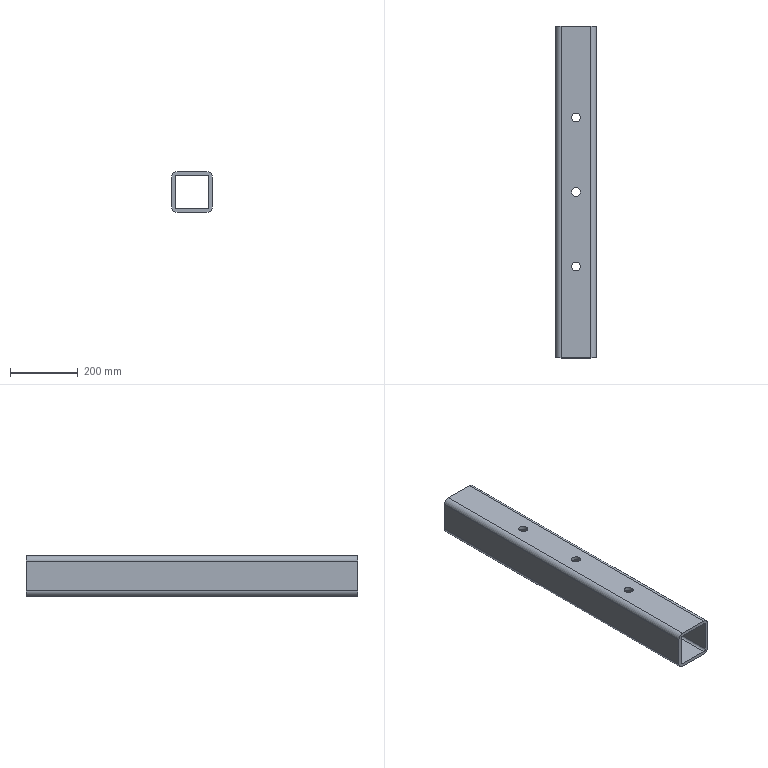Part | SolidWorks | features HoleWzd 1, WeldMemberFeat 1, WeldmentFeature 1 | 1 solid | 30 faces | box 120 x 980 x 120 mm | volume 4095072 mm3 | cylinder 20 | plane 10 | commonest cylinder face diameters 26 x12 12 x4 32 x4
STEP:
#1=CARTESIAN_POINT('',(13.,710.,50.));
#2=VERTEX_POINT('',#1);
#3=CARTESIAN_POINT('',(-13.,710.,50.));
#4=VERTEX_POINT('',#3);
#5=CARTESIAN_POINT('',(0.,710.,50.));
#6=DIRECTION('',(0.,0.,-1.));
#7=DIRECTION('',(-1.,0.,0.));
#8=AXIS2_PLACEMENT_3D('',#5,#6,#7);
#9=CIRCLE('',#8,13.);
#10=EDGE_CURVE('',#2,#4,#9,.T.);
#11=ORIENTED_EDGE('',*,*,#10,.T.);
#12=CARTESIAN_POINT('',(-13.,710.,60.));
#13=VERTEX_POINT('',#12);
#14=CARTESIAN_POINT('',(-13.,710.,60.));
#15=DIRECTION('',(0.,0.,1.));
#16=VECTOR('',#15,1000.);
#17=LINE('',#14,#16);
#18=EDGE_CURVE('',#4,#13,#17,.T.);
#19=ORIENTED_EDGE('',*,*,#18,.T.);
#20=CARTESIAN_POINT('',(13.,710.,60.));
#21=VERTEX_POINT('',#20);
#22=CARTESIAN_POINT('',(0.,710.,60.));
#23=DIRECTION('',(0.,0.,1.));
#24=DIRECTION('',(1.,0.,0.));
#25=AXIS2_PLACEMENT_3D('',#22,#23,#24);
#26=CIRCLE('',#25,13.);
#27=EDGE_CURVE('',#13,#21,#26,.T.);
#28=ORIENTED_EDGE('',*,*,#27,.T.);
#29=CARTESIAN_POINT('',(13.,710.,60.));
#30=DIRECTION('',(0.,0.,1.));
#31=VECTOR('',#30,1000.);
#32=LINE('',#29,#31);
#33=EDGE_CURVE('',#2,#21,#32,.T.);
#34=ORIENTED_EDGE('',*,*,#33,.F.);
#35=EDGE_LOOP('',(#11,#19,#28,#34));
#36=FACE_OUTER_BOUND('',#35,.T.);
#37=CARTESIAN_POINT('',(0.,710.,60.));
#38=DIRECTION('',(0.,0.,1.));
#39=DIRECTION('',(1.,0.,0.));
#40=AXIS2_PLACEMENT_3D('',#37,#38,#39);
#41=CYLINDRICAL_SURFACE('',#40,13.);
#42=ADVANCED_FACE('',(#36),#41,.F.);
#43=CARTESIAN_POINT('',(13.,710.,-60.));
#44=VERTEX_POINT('',#43);
#45=CARTESIAN_POINT('',(-13.,710.,-60.));
#46=VERTEX_POINT('',#45);
#47=CARTESIAN_POINT('',(0.,710.,-60.));
#48=DIRECTION('',(0.,0.,-1.));
#49=DIRECTION('',(1.,0.,0.));
#50=AXIS2_PLACEMENT_3D('',#47,#48,#49);
#51=CIRCLE('',#50,13.);
#52=EDGE_CURVE('',#44,#46,#51,.T.);
#53=ORIENTED_EDGE('',*,*,#52,.T.);
#54=CARTESIAN_POINT('',(-13.,710.,-50.));
#55=VERTEX_POINT('',#54);
#56=CARTESIAN_POINT('',(-13.,710.,60.));
#57=DIRECTION('',(0.,0.,1.));
#58=VECTOR('',#57,1000.);
#59=LINE('',#56,#58);
#60=EDGE_CURVE('',#46,#55,#59,.T.);
#61=ORIENTED_EDGE('',*,*,#60,.T.);
#62=CARTESIAN_POINT('',(13.,710.,-50.));
#63=VERTEX_POINT('',#62);
#64=CARTESIAN_POINT('',(0.,710.,-50.));
#65=DIRECTION('',(0.,0.,1.));
#66=DIRECTION('',(1.,0.,0.));
#67=AXIS2_PLACEMENT_3D('',#64,#65,#66);
#68=CIRCLE('',#67,13.);
#69=EDGE_CURVE('',#55,#63,#68,.T.);
#70=ORIENTED_EDGE('',*,*,#69,.T.);
#71=CARTESIAN_POINT('',(13.,710.,60.));
#72=DIRECTION('',(0.,0.,1.));
#73=VECTOR('',#72,1000.);
#74=LINE('',#71,#73);
#75=EDGE_CURVE('',#44,#63,#74,.T.);
#76=ORIENTED_EDGE('',*,*,#75,.F.);
#77=EDGE_LOOP('',(#53,#61,#70,#76));
#78=FACE_OUTER_BOUND('',#77,.T.);
#79=CARTESIAN_POINT('',(0.,710.,60.));
#80=DIRECTION('',(0.,0.,1.));
#81=DIRECTION('',(1.,0.,0.));
#82=AXIS2_PLACEMENT_3D('',#79,#80,#81);
#83=CYLINDRICAL_SURFACE('',#82,13.);
#84=ADVANCED_FACE('',(#78),#83,.F.);
#85=CARTESIAN_POINT('',(13.,490.,50.));
#86=VERTEX_POINT('',#85);
#87=CARTESIAN_POINT('',(-13.,490.,50.));
#88=VERTEX_POINT('',#87);
#89=CARTESIAN_POINT('',(0.,490.,50.));
#90=DIRECTION('',(0.,0.,-1.));
#91=DIRECTION('',(-1.,0.,0.));
#92=AXIS2_PLACEMENT_3D('',#89,#90,#91);
#93=CIRCLE('',#92,13.);
#94=EDGE_CURVE('',#86,#88,#93,.T.);
#95=ORIENTED_EDGE('',*,*,#94,.T.);
#96=CARTESIAN_POINT('',(-13.,490.,60.));
#97=VERTEX_POINT('',#96);
#98=CARTESIAN_POINT('',(-13.,490.,60.));
#99=DIRECTION('',(0.,0.,1.));
#100=VECTOR('',#99,1000.);
#101=LINE('',#98,#100);
#102=EDGE_CURVE('',#88,#97,#101,.T.);
#103=ORIENTED_EDGE('',*,*,#102,.T.);
#104=CARTESIAN_POINT('',(13.,490.,60.));
#105=VERTEX_POINT('',#104);
#106=CARTESIAN_POINT('',(0.,490.,60.));
#107=DIRECTION('',(0.,0.,1.));
#108=DIRECTION('',(1.,0.,0.));
#109=AXIS2_PLACEMENT_3D('',#106,#107,#108);
#110=CIRCLE('',#109,13.);
#111=EDGE_CURVE('',#97,#105,#110,.T.);
#112=ORIENTED_EDGE('',*,*,#111,.T.);
#113=CARTESIAN_POINT('',(13.,490.,60.));
#114=DIRECTION('',(0.,0.,1.));
#115=VECTOR('',#114,1000.);
#116=LINE('',#113,#115);
#117=EDGE_CURVE('',#86,#105,#116,.T.);
#118=ORIENTED_EDGE('',*,*,#117,.F.);
#119=EDGE_LOOP('',(#95,#103,#112,#118));
#120=FACE_OUTER_BOUND('',#119,.T.);
#121=CARTESIAN_POINT('',(0.,490.,60.));
#122=DIRECTION('',(0.,0.,1.));
#123=DIRECTION('',(1.,0.,0.));
#124=AXIS2_PLACEMENT_3D('',#121,#122,#123);
#125=CYLINDRICAL_SURFACE('',#124,13.);
#126=ADVANCED_FACE('',(#120),#125,.F.);
#127=CARTESIAN_POINT('',(13.,490.,-60.));
#128=VERTEX_POINT('',#127);
#129=CARTESIAN_POINT('',(-13.,490.,-60.));
#130=VERTEX_POINT('',#129);
#131=CARTESIAN_POINT('',(0.,490.,-60.));
#132=DIRECTION('',(0.,0.,-1.));
#133=DIRECTION('',(1.,0.,0.));
#134=AXIS2_PLACEMENT_3D('',#131,#132,#133);
#135=CIRCLE('',#134,13.);
#136=EDGE_CURVE('',#128,#130,#135,.T.);
#137=ORIENTED_EDGE('',*,*,#136,.T.);
#138=CARTESIAN_POINT('',(-13.,490.,-50.));
#139=VERTEX_POINT('',#138);
#140=CARTESIAN_POINT('',(-13.,490.,60.));
#141=DIRECTION('',(0.,0.,1.));
#142=VECTOR('',#141,1000.);
#143=LINE('',#140,#142);
#144=EDGE_CURVE('',#130,#139,#143,.T.);
#145=ORIENTED_EDGE('',*,*,#144,.T.);
#146=CARTESIAN_POINT('',(13.,490.,-50.));
#147=VERTEX_POINT('',#146);
#148=CARTESIAN_POINT('',(0.,490.,-50.));
#149=DIRECTION('',(0.,0.,1.));
#150=DIRECTION('',(1.,0.,0.));
#151=AXIS2_PLACEMENT_3D('',#148,#149,#150);
#152=CIRCLE('',#151,13.);
#153=EDGE_CURVE('',#139,#147,#152,.T.);
#154=ORIENTED_EDGE('',*,*,#153,.T.);
#155=CARTESIAN_POINT('',(13.,490.,60.));
#156=DIRECTION('',(0.,0.,1.));
#157=VECTOR('',#156,1000.);
#158=LINE('',#155,#157);
#159=EDGE_CURVE('',#128,#147,#158,.T.);
#160=ORIENTED_EDGE('',*,*,#159,.F.);
#161=EDGE_LOOP('',(#137,#145,#154,#160));
#162=FACE_OUTER_BOUND('',#161,.T.);
#163=CARTESIAN_POINT('',(0.,490.,60.));
#164=DIRECTION('',(0.,0.,1.));
#165=DIRECTION('',(1.,0.,0.));
#166=AXIS2_PLACEMENT_3D('',#163,#164,#165);
#167=CYLINDRICAL_SURFACE('',#166,13.);
#168=ADVANCED_FACE('',(#162),#167,.F.);
#169=CARTESIAN_POINT('',(13.,270.,50.));
#170=VERTEX_POINT('',#169);
#171=CARTESIAN_POINT('',(-13.,270.,50.));
#172=VERTEX_POINT('',#171);
#173=CARTESIAN_POINT('',(0.,270.,50.));
#174=DIRECTION('',(0.,0.,-1.));
#175=DIRECTION('',(-1.,0.,0.));
#176=AXIS2_PLACEMENT_3D('',#173,#174,#175);
#177=CIRCLE('',#176,13.);
#178=EDGE_CURVE('',#170,#172,#177,.T.);
#179=ORIENTED_EDGE('',*,*,#178,.T.);
#180=CARTESIAN_POINT('',(-13.,270.,60.));
#181=VERTEX_POINT('',#180);
#182=CARTESIAN_POINT('',(-13.,270.,60.));
#183=DIRECTION('',(0.,0.,1.));
#184=VECTOR('',#183,1000.);
#185=LINE('',#182,#184);
#186=EDGE_CURVE('',#172,#181,#185,.T.);
#187=ORIENTED_EDGE('',*,*,#186,.T.);
#188=CARTESIAN_POINT('',(13.,270.,60.));
#189=VERTEX_POINT('',#188);
#190=CARTESIAN_POINT('',(0.,270.,60.));
#191=DIRECTION('',(0.,0.,1.));
#192=DIRECTION('',(1.,0.,0.));
#193=AXIS2_PLACEMENT_3D('',#190,#191,#192);
#194=CIRCLE('',#193,13.);
#195=EDGE_CURVE('',#181,#189,#194,.T.);
#196=ORIENTED_EDGE('',*,*,#195,.T.);
#197=CARTESIAN_POINT('',(13.,270.,60.));
#198=DIRECTION('',(0.,0.,1.));
#199=VECTOR('',#198,1000.);
#200=LINE('',#197,#199);
#201=EDGE_CURVE('',#170,#189,#200,.T.);
#202=ORIENTED_EDGE('',*,*,#201,.F.);
#203=EDGE_LOOP('',(#179,#187,#196,#202));
#204=FACE_OUTER_BOUND('',#203,.T.);
#205=CARTESIAN_POINT('',(0.,270.,60.));
#206=DIRECTION('',(0.,0.,1.));
#207=DIRECTION('',(1.,0.,0.));
#208=AXIS2_PLACEMENT_3D('',#205,#206,#207);
#209=CYLINDRICAL_SURFACE('',#208,13.);
#210=ADVANCED_FACE('',(#204),#209,.F.);
#211=CARTESIAN_POINT('',(13.,270.,-60.));
#212=VERTEX_POINT('',#211);
#213=CARTESIAN_POINT('',(-13.,270.,-60.));
#214=VERTEX_POINT('',#213);
#215=CARTESIAN_POINT('',(0.,270.,-60.));
#216=DIRECTION('',(0.,0.,-1.));
#217=DIRECTION('',(1.,0.,0.));
#218=AXIS2_PLACEMENT_3D('',#215,#216,#217);
#219=CIRCLE('',#218,13.);
#220=EDGE_CURVE('',#212,#214,#219,.T.);
#221=ORIENTED_EDGE('',*,*,#220,.T.);
#222=CARTESIAN_POINT('',(-13.,270.,-50.));
#223=VERTEX_POINT('',#222);
#224=CARTESIAN_POINT('',(-13.,270.,60.));
#225=DIRECTION('',(0.,0.,1.));
#226=VECTOR('',#225,1000.);
#227=LINE('',#224,#226);
#228=EDGE_CURVE('',#214,#223,#227,.T.);
#229=ORIENTED_EDGE('',*,*,#228,.T.);
#230=CARTESIAN_POINT('',(13.,270.,-50.));
#231=VERTEX_POINT('',#230);
#232=CARTESIAN_POINT('',(0.,270.,-50.));
#233=DIRECTION('',(0.,0.,1.));
#234=DIRECTION('',(1.,0.,0.));
#235=AXIS2_PLACEMENT_3D('',#232,#233,#234);
#236=CIRCLE('',#235,13.);
#237=EDGE_CURVE('',#223,#231,#236,.T.);
#238=ORIENTED_EDGE('',*,*,#237,.T.);
#239=CARTESIAN_POINT('',(13.,270.,60.));
#240=DIRECTION('',(0.,0.,1.));
#241=VECTOR('',#240,1000.);
#242=LINE('',#239,#241);
#243=EDGE_CURVE('',#212,#231,#242,.T.);
#244=ORIENTED_EDGE('',*,*,#243,.F.);
#245=EDGE_LOOP('',(#221,#229,#238,#244));
#246=FACE_OUTER_BOUND('',#245,.T.);
#247=CARTESIAN_POINT('',(0.,270.,60.));
#248=DIRECTION('',(0.,0.,1.));
#249=DIRECTION('',(1.,0.,0.));
#250=AXIS2_PLACEMENT_3D('',#247,#248,#249);
#251=CYLINDRICAL_SURFACE('',#250,13.);
#252=ADVANCED_FACE('',(#246),#251,.F.);
#253=ORIENTED_EDGE('',*,*,#136,.F.);
#254=CARTESIAN_POINT('',(0.,490.,-60.));
#255=DIRECTION('',(0.,0.,-1.));
#256=DIRECTION('',(1.,0.,0.));
#257=AXIS2_PLACEMENT_3D('',#254,#255,#256);
#258=CIRCLE('',#257,13.);
#259=EDGE_CURVE('',#130,#128,#258,.T.);
#260=ORIENTED_EDGE('',*,*,#259,.F.);
#261=EDGE_LOOP('',(#253,#260));
#262=FACE_BOUND('',#261,.T.);
#263=ORIENTED_EDGE('',*,*,#220,.F.);
#264=CARTESIAN_POINT('',(0.,270.,-60.));
#265=DIRECTION('',(0.,0.,-1.));
#266=DIRECTION('',(1.,0.,0.));
#267=AXIS2_PLACEMENT_3D('',#264,#265,#266);
#268=CIRCLE('',#267,13.);
#269=EDGE_CURVE('',#214,#212,#268,.T.);
#270=ORIENTED_EDGE('',*,*,#269,.F.);
#271=EDGE_LOOP('',(#263,#270));
#272=FACE_BOUND('',#271,.T.);
#273=CARTESIAN_POINT('',(44.,0.,-60.));
#274=VERTEX_POINT('',#273);
#275=CARTESIAN_POINT('',(-44.,0.,-60.));
#276=VERTEX_POINT('',#275);
#277=CARTESIAN_POINT('',(44.,0.,-60.));
#278=DIRECTION('',(-1.,0.,0.));
#279=VECTOR('',#278,1000.);
#280=LINE('',#277,#279);
#281=EDGE_CURVE('',#274,#276,#280,.T.);
#282=ORIENTED_EDGE('',*,*,#281,.T.);
#283=CARTESIAN_POINT('',(-44.,980.,-60.));
#284=VERTEX_POINT('',#283);
#285=CARTESIAN_POINT('',(-44.,980.,-60.));
#286=DIRECTION('',(0.,-1.,0.));
#287=VECTOR('',#286,1000.);
#288=LINE('',#285,#287);
#289=EDGE_CURVE('',#284,#276,#288,.T.);
#290=ORIENTED_EDGE('',*,*,#289,.F.);
#291=CARTESIAN_POINT('',(44.,980.,-60.));
#292=VERTEX_POINT('',#291);
#293=CARTESIAN_POINT('',(44.,980.,-60.));
#294=DIRECTION('',(-1.,0.,0.));
#295=VECTOR('',#294,1000.);
#296=LINE('',#293,#295);
#297=EDGE_CURVE('',#292,#284,#296,.T.);
#298=ORIENTED_EDGE('',*,*,#297,.F.);
#299=CARTESIAN_POINT('',(44.,980.,-60.));
#300=DIRECTION('',(0.,-1.,0.));
#301=VECTOR('',#300,1000.);
#302=LINE('',#299,#301);
#303=EDGE_CURVE('',#292,#274,#302,.T.);
#304=ORIENTED_EDGE('',*,*,#303,.T.);
#305=EDGE_LOOP('',(#282,#290,#298,#304));
#306=FACE_OUTER_BOUND('',#305,.T.);
#307=ORIENTED_EDGE('',*,*,#52,.F.);
#308=CARTESIAN_POINT('',(0.,710.,-60.));
#309=DIRECTION('',(0.,0.,-1.));
#310=DIRECTION('',(1.,0.,0.));
#311=AXIS2_PLACEMENT_3D('',#308,#309,#310);
#312=CIRCLE('',#311,13.);
#313=EDGE_CURVE('',#46,#44,#312,.T.);
#314=ORIENTED_EDGE('',*,*,#313,.F.);
#315=EDGE_LOOP('',(#307,#314));
#316=FACE_BOUND('',#315,.T.);
#317=CARTESIAN_POINT('',(44.,980.,-60.));
#318=DIRECTION('',(0.,0.,1.));
#319=DIRECTION('',(1.,0.,0.));
#320=AXIS2_PLACEMENT_3D('',#317,#318,#319);
#321=PLANE('',#320);
#322=ADVANCED_FACE('',(#262,#272,#306,#316),#321,.F.);
#323=CARTESIAN_POINT('',(-60.,0.,44.));
#324=VERTEX_POINT('',#323);
#325=CARTESIAN_POINT('',(-44.,0.,60.));
#326=VERTEX_POINT('',#325);
#327=CARTESIAN_POINT('',(-44.,0.,44.));
#328=DIRECTION('',(0.,1.,0.));
#329=DIRECTION('',(0.,0.,1.));
#330=AXIS2_PLACEMENT_3D('',#327,#328,#329);
#331=CIRCLE('',#330,16.);
#332=EDGE_CURVE('',#324,#326,#331,.T.);
#333=ORIENTED_EDGE('',*,*,#332,.T.);
#334=CARTESIAN_POINT('',(-44.,980.,60.));
#335=VERTEX_POINT('',#334);
#336=CARTESIAN_POINT('',(-44.,980.,60.));
#337=DIRECTION('',(0.,-1.,0.));
#338=VECTOR('',#337,1000.);
#339=LINE('',#336,#338);
#340=EDGE_CURVE('',#335,#326,#339,.T.);
#341=ORIENTED_EDGE('',*,*,#340,.F.);
#342=CARTESIAN_POINT('',(-60.,980.,44.));
#343=VERTEX_POINT('',#342);
#344=CARTESIAN_POINT('',(-44.,980.,44.));
#345=DIRECTION('',(0.,1.,0.));
#346=DIRECTION('',(0.,0.,1.));
#347=AXIS2_PLACEMENT_3D('',#344,#345,#346);
#348=CIRCLE('',#347,16.);
#349=EDGE_CURVE('',#343,#335,#348,.T.);
#350=ORIENTED_EDGE('',*,*,#349,.F.);
#351=CARTESIAN_POINT('',(-60.,980.,44.));
#352=DIRECTION('',(0.,-1.,0.));
#353=VECTOR('',#352,1000.);
#354=LINE('',#351,#353);
#355=EDGE_CURVE('',#343,#324,#354,.T.);
#356=ORIENTED_EDGE('',*,*,#355,.T.);
#357=EDGE_LOOP('',(#333,#341,#350,#356));
#358=FACE_OUTER_BOUND('',#357,.T.);
#359=CARTESIAN_POINT('',(-44.,980.,44.));
#360=DIRECTION('',(0.,-1.,0.));
#361=DIRECTION('',(0.,0.,-1.));
#362=AXIS2_PLACEMENT_3D('',#359,#360,#361);
#363=CYLINDRICAL_SURFACE('',#362,16.);
#364=ADVANCED_FACE('',(#358),#363,.T.);
#365=CARTESIAN_POINT('',(0.,710.,60.));
#366=DIRECTION('',(0.,0.,1.));
#367=DIRECTION('',(1.,0.,0.));
#368=AXIS2_PLACEMENT_3D('',#365,#366,#367);
#369=CIRCLE('',#368,13.);
#370=EDGE_CURVE('',#21,#13,#369,.T.);
#371=ORIENTED_EDGE('',*,*,#370,.F.);
#372=ORIENTED_EDGE('',*,*,#27,.F.);
#373=EDGE_LOOP('',(#371,#372));
#374=FACE_BOUND('',#373,.T.);
#375=CARTESIAN_POINT('',(0.,490.,60.));
#376=DIRECTION('',(0.,0.,1.));
#377=DIRECTION('',(1.,0.,0.));
#378=AXIS2_PLACEMENT_3D('',#375,#376,#377);
#379=CIRCLE('',#378,13.);
#380=EDGE_CURVE('',#105,#97,#379,.T.);
#381=ORIENTED_EDGE('',*,*,#380,.F.);
#382=ORIENTED_EDGE('',*,*,#111,.F.);
#383=EDGE_LOOP('',(#381,#382));
#384=FACE_BOUND('',#383,.T.);
#385=CARTESIAN_POINT('',(0.,270.,60.));
#386=DIRECTION('',(0.,0.,1.));
#387=DIRECTION('',(1.,0.,0.));
#388=AXIS2_PLACEMENT_3D('',#385,#386,#387);
#389=CIRCLE('',#388,13.);
#390=EDGE_CURVE('',#189,#181,#389,.T.);
#391=ORIENTED_EDGE('',*,*,#390,.F.);
#392=ORIENTED_EDGE('',*,*,#195,.F.);
#393=EDGE_LOOP('',(#391,#392));
#394=FACE_BOUND('',#393,.T.);
#395=CARTESIAN_POINT('',(44.,0.,60.));
#396=VERTEX_POINT('',#395);
#397=CARTESIAN_POINT('',(-44.,0.,60.));
#398=DIRECTION('',(1.,0.,0.));
#399=VECTOR('',#398,1000.);
#400=LINE('',#397,#399);
#401=EDGE_CURVE('',#326,#396,#400,.T.);
#402=ORIENTED_EDGE('',*,*,#401,.T.);
#403=CARTESIAN_POINT('',(44.,980.,60.));
#404=VERTEX_POINT('',#403);
#405=CARTESIAN_POINT('',(44.,980.,60.));
#406=DIRECTION('',(0.,-1.,0.));
#407=VECTOR('',#406,1000.);
#408=LINE('',#405,#407);
#409=EDGE_CURVE('',#404,#396,#408,.T.);
#410=ORIENTED_EDGE('',*,*,#409,.F.);
#411=CARTESIAN_POINT('',(-44.,980.,60.));
#412=DIRECTION('',(1.,0.,0.));
#413=VECTOR('',#412,1000.);
#414=LINE('',#411,#413);
#415=EDGE_CURVE('',#335,#404,#414,.T.);
#416=ORIENTED_EDGE('',*,*,#415,.F.);
#417=ORIENTED_EDGE('',*,*,#340,.T.);
#418=EDGE_LOOP('',(#402,#410,#416,#417));
#419=FACE_OUTER_BOUND('',#418,.T.);
#420=CARTESIAN_POINT('',(-44.,980.,60.));
#421=DIRECTION('',(0.,0.,-1.));
#422=DIRECTION('',(-1.,0.,0.));
#423=AXIS2_PLACEMENT_3D('',#420,#421,#422);
#424=PLANE('',#423);
#425=ADVANCED_FACE('',(#374,#384,#394,#419),#424,.F.);
#426=CARTESIAN_POINT('',(60.,0.,44.));
#427=VERTEX_POINT('',#426);
#428=CARTESIAN_POINT('',(44.,0.,44.));
#429=DIRECTION('',(0.,1.,0.));
#430=DIRECTION('',(0.,0.,1.));
#431=AXIS2_PLACEMENT_3D('',#428,#429,#430);
#432=CIRCLE('',#431,16.);
#433=EDGE_CURVE('',#396,#427,#432,.T.);
#434=ORIENTED_EDGE('',*,*,#433,.T.);
#435=CARTESIAN_POINT('',(60.,980.,44.));
#436=VERTEX_POINT('',#435);
#437=CARTESIAN_POINT('',(60.,980.,44.));
#438=DIRECTION('',(0.,-1.,0.));
#439=VECTOR('',#438,1000.);
#440=LINE('',#437,#439);
#441=EDGE_CURVE('',#436,#427,#440,.T.);
#442=ORIENTED_EDGE('',*,*,#441,.F.);
#443=CARTESIAN_POINT('',(44.,980.,44.));
#444=DIRECTION('',(0.,1.,0.));
#445=DIRECTION('',(0.,0.,1.));
#446=AXIS2_PLACEMENT_3D('',#443,#444,#445);
#447=CIRCLE('',#446,16.);
#448=EDGE_CURVE('',#404,#436,#447,.T.);
#449=ORIENTED_EDGE('',*,*,#448,.F.);
#450=ORIENTED_EDGE('',*,*,#409,.T.);
#451=EDGE_LOOP('',(#434,#442,#449,#450));
#452=FACE_OUTER_BOUND('',#451,.T.);
#453=CARTESIAN_POINT('',(44.,980.,44.));
#454=DIRECTION('',(0.,-1.,0.));
#455=DIRECTION('',(0.,0.,-1.));
#456=AXIS2_PLACEMENT_3D('',#453,#454,#455);
#457=CYLINDRICAL_SURFACE('',#456,16.);
#458=ADVANCED_FACE('',(#452),#457,.T.);
#459=CARTESIAN_POINT('',(60.,0.,-44.));
#460=VERTEX_POINT('',#459);
#461=CARTESIAN_POINT('',(60.,0.,-44.));
#462=DIRECTION('',(0.,0.,-1.));
#463=VECTOR('',#462,1000.);
#464=LINE('',#461,#463);
#465=EDGE_CURVE('',#427,#460,#464,.T.);
#466=ORIENTED_EDGE('',*,*,#465,.T.);
#467=CARTESIAN_POINT('',(60.,980.,-44.));
#468=VERTEX_POINT('',#467);
#469=CARTESIAN_POINT('',(60.,980.,-44.));
#470=DIRECTION('',(0.,-1.,0.));
#471=VECTOR('',#470,1000.);
#472=LINE('',#469,#471);
#473=EDGE_CURVE('',#468,#460,#472,.T.);
#474=ORIENTED_EDGE('',*,*,#473,.F.);
#475=CARTESIAN_POINT('',(60.,980.,-44.));
#476=DIRECTION('',(0.,0.,-1.));
#477=VECTOR('',#476,1000.);
#478=LINE('',#475,#477);
#479=EDGE_CURVE('',#436,#468,#478,.T.);
#480=ORIENTED_EDGE('',*,*,#479,.F.);
#481=ORIENTED_EDGE('',*,*,#441,.T.);
#482=EDGE_LOOP('',(#466,#474,#480,#481));
#483=FACE_OUTER_BOUND('',#482,.T.);
#484=CARTESIAN_POINT('',(60.,980.,-44.));
#485=DIRECTION('',(-1.,0.,0.));
#486=DIRECTION('',(0.,0.,1.));
#487=AXIS2_PLACEMENT_3D('',#484,#485,#486);
#488=PLANE('',#487);
#489=ADVANCED_FACE('',(#483),#488,.F.);
#490=CARTESIAN_POINT('',(44.,0.,-44.));
#491=DIRECTION('',(0.,1.,0.));
#492=DIRECTION('',(0.,0.,1.));
#493=AXIS2_PLACEMENT_3D('',#490,#491,#492);
#494=CIRCLE('',#493,16.);
#495=EDGE_CURVE('',#460,#274,#494,.T.);
#496=ORIENTED_EDGE('',*,*,#495,.T.);
#497=ORIENTED_EDGE('',*,*,#303,.F.);
#498=CARTESIAN_POINT('',(44.,980.,-44.));
#499=DIRECTION('',(0.,1.,0.));
#500=DIRECTION('',(0.,0.,1.));
#501=AXIS2_PLACEMENT_3D('',#498,#499,#500);
#502=CIRCLE('',#501,16.);
#503=EDGE_CURVE('',#468,#292,#502,.T.);
#504=ORIENTED_EDGE('',*,*,#503,.F.);
#505=ORIENTED_EDGE('',*,*,#473,.T.);
#506=EDGE_LOOP('',(#496,#497,#504,#505));
#507=FACE_OUTER_BOUND('',#506,.T.);
#508=CARTESIAN_POINT('',(44.,980.,-44.));
#509=DIRECTION('',(0.,-1.,0.));
#510=DIRECTION('',(0.,0.,-1.));
#511=AXIS2_PLACEMENT_3D('',#508,#509,#510);
#512=CYLINDRICAL_SURFACE('',#511,16.);
#513=ADVANCED_FACE('',(#507),#512,.T.);
#514=CARTESIAN_POINT('',(-60.,0.,-44.));
#515=VERTEX_POINT('',#514);
#516=CARTESIAN_POINT('',(-44.,0.,-44.));
#517=DIRECTION('',(0.,1.,0.));
#518=DIRECTION('',(0.,0.,1.));
#519=AXIS2_PLACEMENT_3D('',#516,#517,#518);
#520=CIRCLE('',#519,16.);
#521=EDGE_CURVE('',#276,#515,#520,.T.);
#522=ORIENTED_EDGE('',*,*,#521,.T.);
#523=CARTESIAN_POINT('',(-60.,980.,-44.));
#524=VERTEX_POINT('',#523);
#525=CARTESIAN_POINT('',(-60.,980.,-44.));
#526=DIRECTION('',(0.,-1.,0.));
#527=VECTOR('',#526,1000.);
#528=LINE('',#525,#527);
#529=EDGE_CURVE('',#524,#515,#528,.T.);
#530=ORIENTED_EDGE('',*,*,#529,.F.);
#531=CARTESIAN_POINT('',(-44.,980.,-44.));
#532=DIRECTION('',(0.,1.,0.));
#533=DIRECTION('',(0.,0.,1.));
#534=AXIS2_PLACEMENT_3D('',#531,#532,#533);
#535=CIRCLE('',#534,16.);
#536=EDGE_CURVE('',#284,#524,#535,.T.);
#537=ORIENTED_EDGE('',*,*,#536,.F.);
#538=ORIENTED_EDGE('',*,*,#289,.T.);
#539=EDGE_LOOP('',(#522,#530,#537,#538));
#540=FACE_OUTER_BOUND('',#539,.T.);
#541=CARTESIAN_POINT('',(-44.,980.,-44.));
#542=DIRECTION('',(0.,-1.,0.));
#543=DIRECTION('',(0.,0.,-1.));
#544=AXIS2_PLACEMENT_3D('',#541,#542,#543);
#545=CYLINDRICAL_SURFACE('',#544,16.);
#546=ADVANCED_FACE('',(#540),#545,.T.);
#547=CARTESIAN_POINT('',(44.,0.,50.));
#548=VERTEX_POINT('',#547);
#549=CARTESIAN_POINT('',(50.,0.,44.));
#550=VERTEX_POINT('',#549);
#551=CARTESIAN_POINT('',(44.,0.,44.));
#552=DIRECTION('',(0.,1.,0.));
#553=DIRECTION('',(0.,0.,1.));
#554=AXIS2_PLACEMENT_3D('',#551,#552,#553);
#555=CIRCLE('',#554,6.);
#556=EDGE_CURVE('',#548,#550,#555,.T.);
#557=ORIENTED_EDGE('',*,*,#556,.F.);
#558=CARTESIAN_POINT('',(44.,980.,50.));
#559=VERTEX_POINT('',#558);
#560=CARTESIAN_POINT('',(44.,980.,50.));
#561=DIRECTION('',(0.,-1.,0.));
#562=VECTOR('',#561,1000.);
#563=LINE('',#560,#562);
#564=EDGE_CURVE('',#559,#548,#563,.T.);
#565=ORIENTED_EDGE('',*,*,#564,.F.);
#566=CARTESIAN_POINT('',(50.,980.,44.));
#567=VERTEX_POINT('',#566);
#568=CARTESIAN_POINT('',(44.,980.,44.));
#569=DIRECTION('',(0.,1.,0.));
#570=DIRECTION('',(0.,0.,1.));
#571=AXIS2_PLACEMENT_3D('',#568,#569,#570);
#572=CIRCLE('',#571,6.);
#573=EDGE_CURVE('',#559,#567,#572,.T.);
#574=ORIENTED_EDGE('',*,*,#573,.T.);
#575=CARTESIAN_POINT('',(50.,980.,44.));
#576=DIRECTION('',(0.,-1.,0.));
#577=VECTOR('',#576,1000.);
#578=LINE('',#575,#577);
#579=EDGE_CURVE('',#567,#550,#578,.T.);
#580=ORIENTED_EDGE('',*,*,#579,.T.);
#581=EDGE_LOOP('',(#557,#565,#574,#580));
#582=FACE_OUTER_BOUND('',#581,.T.);
#583=CARTESIAN_POINT('',(44.,980.,44.));
#584=DIRECTION('',(0.,-1.,0.));
#585=DIRECTION('',(0.,0.,-1.));
#586=AXIS2_PLACEMENT_3D('',#583,#584,#585);
#587=CYLINDRICAL_SURFACE('',#586,6.);
#588=ADVANCED_FACE('',(#582),#587,.F.);
#589=ORIENTED_EDGE('',*,*,#10,.F.);
#590=CARTESIAN_POINT('',(0.,710.,50.));
#591=DIRECTION('',(0.,0.,-1.));
#592=DIRECTION('',(-1.,0.,0.));
#593=AXIS2_PLACEMENT_3D('',#590,#591,#592);
#594=CIRCLE('',#593,13.);
#595=EDGE_CURVE('',#4,#2,#594,.T.);
#596=ORIENTED_EDGE('',*,*,#595,.F.);
#597=EDGE_LOOP('',(#589,#596));
#598=FACE_BOUND('',#597,.T.);
#599=ORIENTED_EDGE('',*,*,#94,.F.);
#600=CARTESIAN_POINT('',(0.,490.,50.));
#601=DIRECTION('',(0.,0.,-1.));
#602=DIRECTION('',(-1.,0.,0.));
#603=AXIS2_PLACEMENT_3D('',#600,#601,#602);
#604=CIRCLE('',#603,13.);
#605=EDGE_CURVE('',#88,#86,#604,.T.);
#606=ORIENTED_EDGE('',*,*,#605,.F.);
#607=EDGE_LOOP('',(#599,#606));
#608=FACE_BOUND('',#607,.T.);
#609=ORIENTED_EDGE('',*,*,#178,.F.);
#610=CARTESIAN_POINT('',(0.,270.,50.));
#611=DIRECTION('',(0.,0.,-1.));
#612=DIRECTION('',(-1.,0.,0.));
#613=AXIS2_PLACEMENT_3D('',#610,#611,#612);
#614=CIRCLE('',#613,13.);
#615=EDGE_CURVE('',#172,#170,#614,.T.);
#616=ORIENTED_EDGE('',*,*,#615,.F.);
#617=EDGE_LOOP('',(#609,#616));
#618=FACE_BOUND('',#617,.T.);
#619=CARTESIAN_POINT('',(-44.,0.,50.));
#620=VERTEX_POINT('',#619);
#621=CARTESIAN_POINT('',(-44.,0.,50.));
#622=DIRECTION('',(1.,0.,0.));
#623=VECTOR('',#622,1000.);
#624=LINE('',#621,#623);
#625=EDGE_CURVE('',#620,#548,#624,.T.);
#626=ORIENTED_EDGE('',*,*,#625,.F.);
#627=CARTESIAN_POINT('',(-44.,980.,50.));
#628=VERTEX_POINT('',#627);
#629=CARTESIAN_POINT('',(-44.,980.,50.));
#630=DIRECTION('',(0.,-1.,0.));
#631=VECTOR('',#630,1000.);
#632=LINE('',#629,#631);
#633=EDGE_CURVE('',#628,#620,#632,.T.);
#634=ORIENTED_EDGE('',*,*,#633,.F.);
#635=CARTESIAN_POINT('',(-44.,980.,50.));
#636=DIRECTION('',(1.,0.,0.));
#637=VECTOR('',#636,1000.);
#638=LINE('',#635,#637);
#639=EDGE_CURVE('',#628,#559,#638,.T.);
#640=ORIENTED_EDGE('',*,*,#639,.T.);
#641=ORIENTED_EDGE('',*,*,#564,.T.);
#642=EDGE_LOOP('',(#626,#634,#640,#641));
#643=FACE_OUTER_BOUND('',#642,.T.);
#644=CARTESIAN_POINT('',(-44.,980.,50.));
#645=DIRECTION('',(0.,0.,-1.));
#646=DIRECTION('',(-1.,0.,0.));
#647=AXIS2_PLACEMENT_3D('',#644,#645,#646);
#648=PLANE('',#647);
#649=ADVANCED_FACE('',(#598,#608,#618,#643),#648,.T.);
#650=CARTESIAN_POINT('',(-50.,0.,44.));
#651=VERTEX_POINT('',#650);
#652=CARTESIAN_POINT('',(-44.,0.,44.));
#653=DIRECTION('',(0.,1.,0.));
#654=DIRECTION('',(0.,0.,1.));
#655=AXIS2_PLACEMENT_3D('',#652,#653,#654);
#656=CIRCLE('',#655,6.);
#657=EDGE_CURVE('',#651,#620,#656,.T.);
#658=ORIENTED_EDGE('',*,*,#657,.F.);
#659=CARTESIAN_POINT('',(-50.,980.,44.));
#660=VERTEX_POINT('',#659);
#661=CARTESIAN_POINT('',(-50.,980.,44.));
#662=DIRECTION('',(0.,-1.,0.));
#663=VECTOR('',#662,1000.);
#664=LINE('',#661,#663);
#665=EDGE_CURVE('',#660,#651,#664,.T.);
#666=ORIENTED_EDGE('',*,*,#665,.F.);
#667=CARTESIAN_POINT('',(-44.,980.,44.));
#668=DIRECTION('',(0.,1.,0.));
#669=DIRECTION('',(0.,0.,1.));
#670=AXIS2_PLACEMENT_3D('',#667,#668,#669);
#671=CIRCLE('',#670,6.);
#672=EDGE_CURVE('',#660,#628,#671,.T.);
#673=ORIENTED_EDGE('',*,*,#672,.T.);
#674=ORIENTED_EDGE('',*,*,#633,.T.);
#675=EDGE_LOOP('',(#658,#666,#673,#674));
#676=FACE_OUTER_BOUND('',#675,.T.);
#677=CARTESIAN_POINT('',(-44.,980.,44.));
#678=DIRECTION('',(0.,-1.,0.));
#679=DIRECTION('',(0.,0.,-1.));
#680=AXIS2_PLACEMENT_3D('',#677,#678,#679);
#681=CYLINDRICAL_SURFACE('',#680,6.);
#682=ADVANCED_FACE('',(#676),#681,.F.);
#683=CARTESIAN_POINT('',(-50.,0.,-44.));
#684=VERTEX_POINT('',#683);
#685=CARTESIAN_POINT('',(-50.,0.,44.));
#686=DIRECTION('',(0.,0.,1.));
#687=VECTOR('',#686,1000.);
#688=LINE('',#685,#687);
#689=EDGE_CURVE('',#684,#651,#688,.T.);
#690=ORIENTED_EDGE('',*,*,#689,.F.);
#691=CARTESIAN_POINT('',(-50.,980.,-44.));
#692=VERTEX_POINT('',#691);
#693=CARTESIAN_POINT('',(-50.,980.,-44.));
#694=DIRECTION('',(0.,-1.,0.));
#695=VECTOR('',#694,1000.);
#696=LINE('',#693,#695);
#697=EDGE_CURVE('',#692,#684,#696,.T.);
#698=ORIENTED_EDGE('',*,*,#697,.F.);
#699=CARTESIAN_POINT('',(-50.,980.,44.));
#700=DIRECTION('',(0.,0.,1.));
#701=VECTOR('',#700,1000.);
#702=LINE('',#699,#701);
#703=EDGE_CURVE('',#692,#660,#702,.T.);
#704=ORIENTED_EDGE('',*,*,#703,.T.);
#705=ORIENTED_EDGE('',*,*,#665,.T.);
#706=EDGE_LOOP('',(#690,#698,#704,#705));
#707=FACE_OUTER_BOUND('',#706,.T.);
#708=CARTESIAN_POINT('',(-50.,980.,44.));
#709=DIRECTION('',(1.,0.,0.));
#710=DIRECTION('',(0.,0.,-1.));
#711=AXIS2_PLACEMENT_3D('',#708,#709,#710);
#712=PLANE('',#711);
#713=ADVANCED_FACE('',(#707),#712,.T.);
#714=CARTESIAN_POINT('',(-44.,0.,-50.));
#715=VERTEX_POINT('',#714);
#716=CARTESIAN_POINT('',(-44.,0.,-44.));
#717=DIRECTION('',(0.,1.,0.));
#718=DIRECTION('',(0.,0.,1.));
#719=AXIS2_PLACEMENT_3D('',#716,#717,#718);
#720=CIRCLE('',#719,6.);
#721=EDGE_CURVE('',#715,#684,#720,.T.);
#722=ORIENTED_EDGE('',*,*,#721,.F.);
#723=CARTESIAN_POINT('',(-44.,980.,-50.));
#724=VERTEX_POINT('',#723);
#725=CARTESIAN_POINT('',(-44.,980.,-50.));
#726=DIRECTION('',(0.,-1.,0.));
#727=VECTOR('',#726,1000.);
#728=LINE('',#725,#727);
#729=EDGE_CURVE('',#724,#715,#728,.T.);
#730=ORIENTED_EDGE('',*,*,#729,.F.);
#731=CARTESIAN_POINT('',(-44.,980.,-44.));
#732=DIRECTION('',(0.,1.,0.));
#733=DIRECTION('',(0.,0.,1.));
#734=AXIS2_PLACEMENT_3D('',#731,#732,#733);
#735=CIRCLE('',#734,6.);
#736=EDGE_CURVE('',#724,#692,#735,.T.);
#737=ORIENTED_EDGE('',*,*,#736,.T.);
#738=ORIENTED_EDGE('',*,*,#697,.T.);
#739=EDGE_LOOP('',(#722,#730,#737,#738));
#740=FACE_OUTER_BOUND('',#739,.T.);
#741=CARTESIAN_POINT('',(-44.,980.,-44.));
#742=DIRECTION('',(0.,-1.,0.));
#743=DIRECTION('',(0.,0.,-1.));
#744=AXIS2_PLACEMENT_3D('',#741,#742,#743);
#745=CYLINDRICAL_SURFACE('',#744,6.);
#746=ADVANCED_FACE('',(#740),#745,.F.);
#747=CARTESIAN_POINT('',(0.,710.,-50.));
#748=DIRECTION('',(0.,0.,1.));
#749=DIRECTION('',(1.,0.,0.));
#750=AXIS2_PLACEMENT_3D('',#747,#748,#749);
#751=CIRCLE('',#750,13.);
#752=EDGE_CURVE('',#63,#55,#751,.T.);
#753=ORIENTED_EDGE('',*,*,#752,.F.);
#754=ORIENTED_EDGE('',*,*,#69,.F.);
#755=EDGE_LOOP('',(#753,#754));
#756=FACE_BOUND('',#755,.T.);
#757=CARTESIAN_POINT('',(0.,490.,-50.));
#758=DIRECTION('',(0.,0.,1.));
#759=DIRECTION('',(1.,0.,0.));
#760=AXIS2_PLACEMENT_3D('',#757,#758,#759);
#761=CIRCLE('',#760,13.);
#762=EDGE_CURVE('',#147,#139,#761,.T.);
#763=ORIENTED_EDGE('',*,*,#762,.F.);
#764=ORIENTED_EDGE('',*,*,#153,.F.);
#765=EDGE_LOOP('',(#763,#764));
#766=FACE_BOUND('',#765,.T.);
#767=CARTESIAN_POINT('',(0.,270.,-50.));
#768=DIRECTION('',(0.,0.,1.));
#769=DIRECTION('',(1.,0.,0.));
#770=AXIS2_PLACEMENT_3D('',#767,#768,#769);
#771=CIRCLE('',#770,13.);
#772=EDGE_CURVE('',#231,#223,#771,.T.);
#773=ORIENTED_EDGE('',*,*,#772,.F.);
#774=ORIENTED_EDGE('',*,*,#237,.F.);
#775=EDGE_LOOP('',(#773,#774));
#776=FACE_BOUND('',#775,.T.);
#777=CARTESIAN_POINT('',(44.,0.,-50.));
#778=VERTEX_POINT('',#777);
#779=CARTESIAN_POINT('',(44.,0.,-50.));
#780=DIRECTION('',(-1.,0.,0.));
#781=VECTOR('',#780,1000.);
#782=LINE('',#779,#781);
#783=EDGE_CURVE('',#778,#715,#782,.T.);
#784=ORIENTED_EDGE('',*,*,#783,.F.);
#785=CARTESIAN_POINT('',(44.,980.,-50.));
#786=VERTEX_POINT('',#785);
#787=CARTESIAN_POINT('',(44.,980.,-50.));
#788=DIRECTION('',(0.,-1.,0.));
#789=VECTOR('',#788,1000.);
#790=LINE('',#787,#789);
#791=EDGE_CURVE('',#786,#778,#790,.T.);
#792=ORIENTED_EDGE('',*,*,#791,.F.);
#793=CARTESIAN_POINT('',(44.,980.,-50.));
#794=DIRECTION('',(-1.,0.,0.));
#795=VECTOR('',#794,1000.);
#796=LINE('',#793,#795);
#797=EDGE_CURVE('',#786,#724,#796,.T.);
#798=ORIENTED_EDGE('',*,*,#797,.T.);
#799=ORIENTED_EDGE('',*,*,#729,.T.);
#800=EDGE_LOOP('',(#784,#792,#798,#799));
#801=FACE_OUTER_BOUND('',#800,.T.);
#802=CARTESIAN_POINT('',(44.,980.,-50.));
#803=DIRECTION('',(0.,0.,1.));
#804=DIRECTION('',(1.,0.,0.));
#805=AXIS2_PLACEMENT_3D('',#802,#803,#804);
#806=PLANE('',#805);
#807=ADVANCED_FACE('',(#756,#766,#776,#801),#806,.T.);
#808=CARTESIAN_POINT('',(50.,0.,-44.));
#809=VERTEX_POINT('',#808);
#810=CARTESIAN_POINT('',(44.,0.,-44.));
#811=DIRECTION('',(0.,1.,0.));
#812=DIRECTION('',(0.,0.,1.));
#813=AXIS2_PLACEMENT_3D('',#810,#811,#812);
#814=CIRCLE('',#813,6.);
#815=EDGE_CURVE('',#809,#778,#814,.T.);
#816=ORIENTED_EDGE('',*,*,#815,.F.);
#817=CARTESIAN_POINT('',(50.,980.,-44.));
#818=VERTEX_POINT('',#817);
#819=CARTESIAN_POINT('',(50.,980.,-44.));
#820=DIRECTION('',(0.,-1.,0.));
#821=VECTOR('',#820,1000.);
#822=LINE('',#819,#821);
#823=EDGE_CURVE('',#818,#809,#822,.T.);
#824=ORIENTED_EDGE('',*,*,#823,.F.);
#825=CARTESIAN_POINT('',(44.,980.,-44.));
#826=DIRECTION('',(0.,1.,0.));
#827=DIRECTION('',(0.,0.,1.));
#828=AXIS2_PLACEMENT_3D('',#825,#826,#827);
#829=CIRCLE('',#828,6.);
#830=EDGE_CURVE('',#818,#786,#829,.T.);
#831=ORIENTED_EDGE('',*,*,#830,.T.);
#832=ORIENTED_EDGE('',*,*,#791,.T.);
#833=EDGE_LOOP('',(#816,#824,#831,#832));
#834=FACE_OUTER_BOUND('',#833,.T.);
#835=CARTESIAN_POINT('',(44.,980.,-44.));
#836=DIRECTION('',(0.,-1.,0.));
#837=DIRECTION('',(0.,0.,-1.));
#838=AXIS2_PLACEMENT_3D('',#835,#836,#837);
#839=CYLINDRICAL_SURFACE('',#838,6.);
#840=ADVANCED_FACE('',(#834),#839,.F.);
#841=CARTESIAN_POINT('',(50.,0.,-44.));
#842=DIRECTION('',(0.,0.,-1.));
#843=VECTOR('',#842,1000.);
#844=LINE('',#841,#843);
#845=EDGE_CURVE('',#550,#809,#844,.T.);
#846=ORIENTED_EDGE('',*,*,#845,.F.);
#847=ORIENTED_EDGE('',*,*,#579,.F.);
#848=CARTESIAN_POINT('',(50.,980.,-44.));
#849=DIRECTION('',(0.,0.,-1.));
#850=VECTOR('',#849,1000.);
#851=LINE('',#848,#850);
#852=EDGE_CURVE('',#567,#818,#851,.T.);
#853=ORIENTED_EDGE('',*,*,#852,.T.);
#854=ORIENTED_EDGE('',*,*,#823,.T.);
#855=EDGE_LOOP('',(#846,#847,#853,#854));
#856=FACE_OUTER_BOUND('',#855,.T.);
#857=CARTESIAN_POINT('',(50.,980.,-44.));
#858=DIRECTION('',(-1.,0.,0.));
#859=DIRECTION('',(0.,0.,1.));
#860=AXIS2_PLACEMENT_3D('',#857,#858,#859);
#861=PLANE('',#860);
#862=ADVANCED_FACE('',(#856),#861,.T.);
#863=CARTESIAN_POINT('',(-60.,0.,44.));
#864=DIRECTION('',(0.,0.,1.));
#865=VECTOR('',#864,1000.);
#866=LINE('',#863,#865);
#867=EDGE_CURVE('',#515,#324,#866,.T.);
#868=ORIENTED_EDGE('',*,*,#867,.T.);
#869=ORIENTED_EDGE('',*,*,#355,.F.);
#870=CARTESIAN_POINT('',(-60.,980.,44.));
#871=DIRECTION('',(0.,0.,1.));
#872=VECTOR('',#871,1000.);
#873=LINE('',#870,#872);
#874=EDGE_CURVE('',#524,#343,#873,.T.);
#875=ORIENTED_EDGE('',*,*,#874,.F.);
#876=ORIENTED_EDGE('',*,*,#529,.T.);
#877=EDGE_LOOP('',(#868,#869,#875,#876));
#878=FACE_OUTER_BOUND('',#877,.T.);
#879=CARTESIAN_POINT('',(-60.,980.,44.));
#880=DIRECTION('',(1.,0.,0.));
#881=DIRECTION('',(0.,0.,-1.));
#882=AXIS2_PLACEMENT_3D('',#879,#880,#881);
#883=PLANE('',#882);
#884=ADVANCED_FACE('',(#878),#883,.F.);
#885=ORIENTED_EDGE('',*,*,#573,.F.);
#886=ORIENTED_EDGE('',*,*,#639,.F.);
#887=ORIENTED_EDGE('',*,*,#672,.F.);
#888=ORIENTED_EDGE('',*,*,#703,.F.);
#889=ORIENTED_EDGE('',*,*,#736,.F.);
#890=ORIENTED_EDGE('',*,*,#797,.F.);
#891=ORIENTED_EDGE('',*,*,#830,.F.);
#892=ORIENTED_EDGE('',*,*,#852,.F.);
#893=EDGE_LOOP('',(#885,#886,#887,#888,#889,#890,#891,#892));
#894=FACE_BOUND('',#893,.T.);
#895=ORIENTED_EDGE('',*,*,#349,.T.);
#896=ORIENTED_EDGE('',*,*,#415,.T.);
#897=ORIENTED_EDGE('',*,*,#448,.T.);
#898=ORIENTED_EDGE('',*,*,#479,.T.);
#899=ORIENTED_EDGE('',*,*,#503,.T.);
#900=ORIENTED_EDGE('',*,*,#297,.T.);
#901=ORIENTED_EDGE('',*,*,#536,.T.);
#902=ORIENTED_EDGE('',*,*,#874,.T.);
#903=EDGE_LOOP('',(#895,#896,#897,#898,#899,#900,#901,#902));
#904=FACE_OUTER_BOUND('',#903,.T.);
#905=CARTESIAN_POINT('',(-44.,980.,44.));
#906=DIRECTION('',(0.,1.,0.));
#907=DIRECTION('',(0.,0.,1.));
#908=AXIS2_PLACEMENT_3D('',#905,#906,#907);
#909=PLANE('',#908);
#910=ADVANCED_FACE('',(#894,#904),#909,.T.);
#911=ORIENTED_EDGE('',*,*,#556,.T.);
#912=ORIENTED_EDGE('',*,*,#845,.T.);
#913=ORIENTED_EDGE('',*,*,#815,.T.);
#914=ORIENTED_EDGE('',*,*,#783,.T.);
#915=ORIENTED_EDGE('',*,*,#721,.T.);
#916=ORIENTED_EDGE('',*,*,#689,.T.);
#917=ORIENTED_EDGE('',*,*,#657,.T.);
#918=ORIENTED_EDGE('',*,*,#625,.T.);
#919=EDGE_LOOP('',(#911,#912,#913,#914,#915,#916,#917,#918));
#920=FACE_BOUND('',#919,.T.);
#921=ORIENTED_EDGE('',*,*,#332,.F.);
#922=ORIENTED_EDGE('',*,*,#867,.F.);
#923=ORIENTED_EDGE('',*,*,#521,.F.);
#924=ORIENTED_EDGE('',*,*,#281,.F.);
#925=ORIENTED_EDGE('',*,*,#495,.F.);
#926=ORIENTED_EDGE('',*,*,#465,.F.);
#927=ORIENTED_EDGE('',*,*,#433,.F.);
#928=ORIENTED_EDGE('',*,*,#401,.F.);
#929=EDGE_LOOP('',(#921,#922,#923,#924,#925,#926,#927,#928));
#930=FACE_OUTER_BOUND('',#929,.T.);
#931=CARTESIAN_POINT('',(-44.,0.,44.));
#932=DIRECTION('',(0.,1.,0.));
#933=DIRECTION('',(0.,0.,1.));
#934=AXIS2_PLACEMENT_3D('',#931,#932,#933);
#935=PLANE('',#934);
#936=ADVANCED_FACE('',(#920,#930),#935,.F.);
#937=ORIENTED_EDGE('',*,*,#228,.F.);
#938=ORIENTED_EDGE('',*,*,#269,.T.);
#939=ORIENTED_EDGE('',*,*,#243,.T.);
#940=ORIENTED_EDGE('',*,*,#772,.T.);
#941=EDGE_LOOP('',(#937,#938,#939,#940));
#942=FACE_OUTER_BOUND('',#941,.T.);
#943=CARTESIAN_POINT('',(0.,270.,60.));
#944=DIRECTION('',(0.,0.,1.));
#945=DIRECTION('',(1.,0.,0.));
#946=AXIS2_PLACEMENT_3D('',#943,#944,#945);
#947=CYLINDRICAL_SURFACE('',#946,13.);
#948=ADVANCED_FACE('',(#942),#947,.F.);
#949=ORIENTED_EDGE('',*,*,#186,.F.);
#950=ORIENTED_EDGE('',*,*,#615,.T.);
#951=ORIENTED_EDGE('',*,*,#201,.T.);
#952=ORIENTED_EDGE('',*,*,#390,.T.);
#953=EDGE_LOOP('',(#949,#950,#951,#952));
#954=FACE_OUTER_BOUND('',#953,.T.);
#955=CARTESIAN_POINT('',(0.,270.,60.));
#956=DIRECTION('',(0.,0.,1.));
#957=DIRECTION('',(1.,0.,0.));
#958=AXIS2_PLACEMENT_3D('',#955,#956,#957);
#959=CYLINDRICAL_SURFACE('',#958,13.);
#960=ADVANCED_FACE('',(#954),#959,.F.);
#961=ORIENTED_EDGE('',*,*,#144,.F.);
#962=ORIENTED_EDGE('',*,*,#259,.T.);
#963=ORIENTED_EDGE('',*,*,#159,.T.);
#964=ORIENTED_EDGE('',*,*,#762,.T.);
#965=EDGE_LOOP('',(#961,#962,#963,#964));
#966=FACE_OUTER_BOUND('',#965,.T.);
#967=CARTESIAN_POINT('',(0.,490.,60.));
#968=DIRECTION('',(0.,0.,1.));
#969=DIRECTION('',(1.,0.,0.));
#970=AXIS2_PLACEMENT_3D('',#967,#968,#969);
#971=CYLINDRICAL_SURFACE('',#970,13.);
#972=ADVANCED_FACE('',(#966),#971,.F.);
#973=ORIENTED_EDGE('',*,*,#102,.F.);
#974=ORIENTED_EDGE('',*,*,#605,.T.);
#975=ORIENTED_EDGE('',*,*,#117,.T.);
#976=ORIENTED_EDGE('',*,*,#380,.T.);
#977=EDGE_LOOP('',(#973,#974,#975,#976));
#978=FACE_OUTER_BOUND('',#977,.T.);
#979=CARTESIAN_POINT('',(0.,490.,60.));
#980=DIRECTION('',(0.,0.,1.));
#981=DIRECTION('',(1.,0.,0.));
#982=AXIS2_PLACEMENT_3D('',#979,#980,#981);
#983=CYLINDRICAL_SURFACE('',#982,13.);
#984=ADVANCED_FACE('',(#978),#983,.F.);
#985=ORIENTED_EDGE('',*,*,#60,.F.);
#986=ORIENTED_EDGE('',*,*,#313,.T.);
#987=ORIENTED_EDGE('',*,*,#75,.T.);
#988=ORIENTED_EDGE('',*,*,#752,.T.);
#989=EDGE_LOOP('',(#985,#986,#987,#988));
#990=FACE_OUTER_BOUND('',#989,.T.);
#991=CARTESIAN_POINT('',(0.,710.,60.));
#992=DIRECTION('',(0.,0.,1.));
#993=DIRECTION('',(1.,0.,0.));
#994=AXIS2_PLACEMENT_3D('',#991,#992,#993);
#995=CYLINDRICAL_SURFACE('',#994,13.);
#996=ADVANCED_FACE('',(#990),#995,.F.);
#997=ORIENTED_EDGE('',*,*,#18,.F.);
#998=ORIENTED_EDGE('',*,*,#595,.T.);
#999=ORIENTED_EDGE('',*,*,#33,.T.);
#1000=ORIENTED_EDGE('',*,*,#370,.T.);
#1001=EDGE_LOOP('',(#997,#998,#999,#1000));
#1002=FACE_OUTER_BOUND('',#1001,.T.);
#1003=CARTESIAN_POINT('',(0.,710.,60.));
#1004=DIRECTION('',(0.,0.,1.));
#1005=DIRECTION('',(1.,0.,0.));
#1006=AXIS2_PLACEMENT_3D('',#1003,#1004,#1005);
#1007=CYLINDRICAL_SURFACE('',#1006,13.);
#1008=ADVANCED_FACE('',(#1002),#1007,.F.);
#1009=CLOSED_SHELL('',(#42,#84,#126,#168,#210,#252,#322,#364,#425,#458,#489,#513,#546,#588,#649,#682,#713,#746,#807,#840,#862,#884,#910,#936,#948,#960,#972,#984,#996,#1008));
#1010=MANIFOLD_SOLID_BREP('',#1009);
#1011=CARTESIAN_POINT('',(0.,0.,0.));
#1012=DIRECTION('',(0.,0.,1.));
#1013=DIRECTION('',(1.,0.,0.));
#1014=AXIS2_PLACEMENT_3D('',#1011,#1012,#1013);
#1015=(LENGTH_UNIT()NAMED_UNIT(*)SI_UNIT(.MILLI.,.METRE.));
#1016=UNCERTAINTY_MEASURE_WITH_UNIT(LENGTH_MEASURE(0.00001),#1015,'','');
#1017=(NAMED_UNIT(*)PLANE_ANGLE_UNIT()SI_UNIT($,.RADIAN.));
#1018=(NAMED_UNIT(*)SI_UNIT($,.STERADIAN.)SOLID_ANGLE_UNIT());
#1019=(GEOMETRIC_REPRESENTATION_CONTEXT(3)GLOBAL_UNCERTAINTY_ASSIGNED_CONTEXT((#1016))GLOBAL_UNIT_ASSIGNED_CONTEXT((#1015,#1017,#1018))REPRESENTATION_CONTEXT('',''));
#1020=ADVANCED_BREP_SHAPE_REPRESENTATION('',(#1010,#1014),#1019);